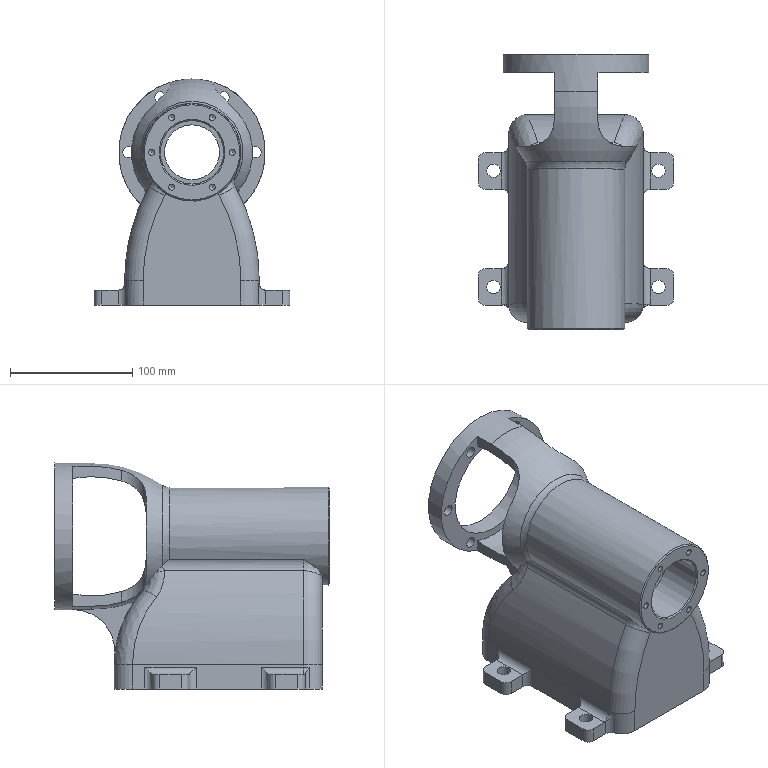Part | NX | features DATUM_CSYS 25, SKETCH 24, EXTRACT_DATUM_AXIS 18, EXTRACT_FACE 18, HOLE PACKAGE 18, SIMPLE HOLE 18, Instance Feature 15, SYMBOLIC_THREAD 12, EXTRUDE 11, REPLACE_FACE 10, BLEND 8, UNITE 7, OFFSET_REGION 4, Pattern Feature 3, CHAMFER 1, CPROJ 1, Container 1, EXTRACT_BODY 1, Geometry Instance 1, SWP104 1, TRIM BODY 1 | 1 solid | 157 faces | box 160 x 225 x 185 mm | volume 973073 mm3 | cylinder 75 | plane 40 | cone 16 | torus 13 | spline 9 | sphere 4 | commonest cylinder face diameters 12 x20 5 x12 20 x8 9 x6 11 x4 30 x4